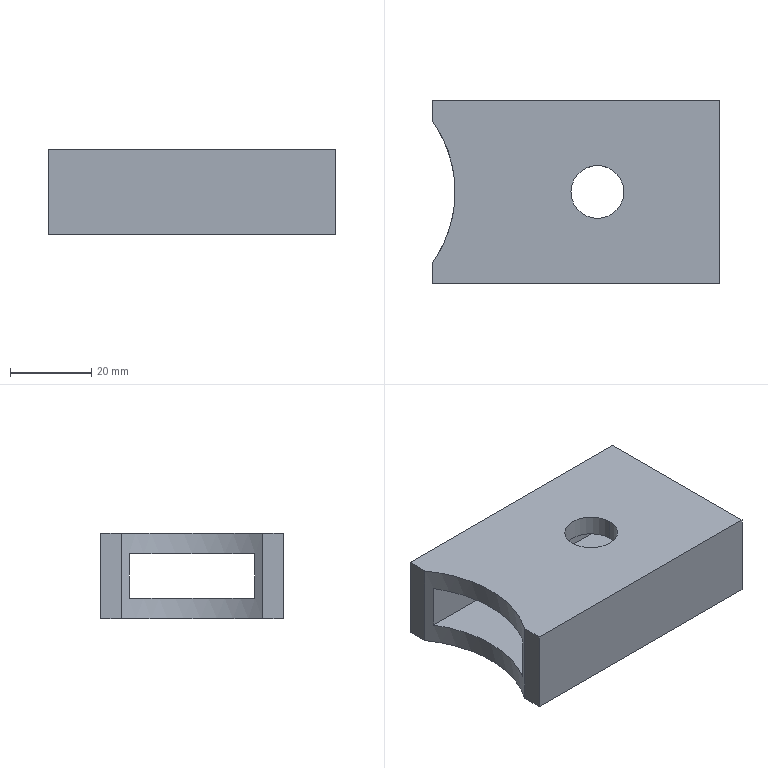Part | SolidWorks | features ICE 3, Extrusion 1 | 1 solid | 20 faces | box 70.526 x 45 x 21 mm | volume 38872 mm3 | plane 17 | cylinder 3 | commonest cylinder face diameters 13 x2 60 x1
STEP:
#1=CARTESIAN_POINT('',(71.5,0.,5.5));
#2=VERTEX_POINT('',#1);
#3=CARTESIAN_POINT('',(58.5,0.,5.5));
#4=VERTEX_POINT('',#3);
#5=CARTESIAN_POINT('',(65.,0.,5.5));
#6=DIRECTION('',(0.,0.,-1.));
#7=DIRECTION('',(0.,-1.,0.));
#8=AXIS2_PLACEMENT_3D('',#5,#6,#7);
#9=CIRCLE('',#8,6.5);
#10=EDGE_CURVE('',#2,#4,#9,.T.);
#11=ORIENTED_EDGE('',*,*,#10,.T.);
#12=CARTESIAN_POINT('',(58.5,0.,10.5));
#13=VERTEX_POINT('',#12);
#14=CARTESIAN_POINT('',(58.5,0.,-10.501));
#15=DIRECTION('',(0.,0.,1.));
#16=VECTOR('',#15,1000.);
#17=LINE('',#14,#16);
#18=EDGE_CURVE('',#4,#13,#17,.T.);
#19=ORIENTED_EDGE('',*,*,#18,.T.);
#20=CARTESIAN_POINT('',(71.5,0.,10.5));
#21=VERTEX_POINT('',#20);
#22=CARTESIAN_POINT('',(65.,0.,10.5));
#23=DIRECTION('',(0.,0.,1.));
#24=DIRECTION('',(1.,0.,0.));
#25=AXIS2_PLACEMENT_3D('',#22,#23,#24);
#26=CIRCLE('',#25,6.5);
#27=EDGE_CURVE('',#13,#21,#26,.T.);
#28=ORIENTED_EDGE('',*,*,#27,.T.);
#29=CARTESIAN_POINT('',(71.5,0.,-10.501));
#30=DIRECTION('',(0.,0.,1.));
#31=VECTOR('',#30,1000.);
#32=LINE('',#29,#31);
#33=EDGE_CURVE('',#2,#21,#32,.T.);
#34=ORIENTED_EDGE('',*,*,#33,.F.);
#35=EDGE_LOOP('',(#11,#19,#28,#34));
#36=FACE_OUTER_BOUND('',#35,.T.);
#37=CARTESIAN_POINT('',(65.,0.,-10.501));
#38=DIRECTION('',(0.,0.,1.));
#39=DIRECTION('',(1.,0.,0.));
#40=AXIS2_PLACEMENT_3D('',#37,#38,#39);
#41=CYLINDRICAL_SURFACE('',#40,6.5);
#42=ADVANCED_FACE('',(#36),#41,.F.);
#43=CARTESIAN_POINT('',(95.,22.5,-10.5));
#44=VERTEX_POINT('',#43);
#45=CARTESIAN_POINT('',(24.474,22.5,-10.5));
#46=VERTEX_POINT('',#45);
#47=CARTESIAN_POINT('',(24.474,22.5,-10.5));
#48=DIRECTION('',(-1.,0.,0.));
#49=VECTOR('',#48,1000.);
#50=LINE('',#47,#49);
#51=EDGE_CURVE('',#44,#46,#50,.T.);
#52=ORIENTED_EDGE('',*,*,#51,.T.);
#53=CARTESIAN_POINT('',(24.474,22.5,10.5));
#54=VERTEX_POINT('',#53);
#55=CARTESIAN_POINT('',(24.474,22.5,10.5));
#56=DIRECTION('',(0.,0.,-1.));
#57=VECTOR('',#56,1000.);
#58=LINE('',#55,#57);
#59=EDGE_CURVE('',#54,#46,#58,.T.);
#60=ORIENTED_EDGE('',*,*,#59,.F.);
#61=CARTESIAN_POINT('',(95.,22.5,10.5));
#62=VERTEX_POINT('',#61);
#63=CARTESIAN_POINT('',(24.474,22.5,10.5));
#64=DIRECTION('',(-1.,0.,0.));
#65=VECTOR('',#64,1000.);
#66=LINE('',#63,#65);
#67=EDGE_CURVE('',#62,#54,#66,.T.);
#68=ORIENTED_EDGE('',*,*,#67,.F.);
#69=CARTESIAN_POINT('',(95.,22.5,10.5));
#70=DIRECTION('',(0.,0.,-1.));
#71=VECTOR('',#70,1000.);
#72=LINE('',#69,#71);
#73=EDGE_CURVE('',#62,#44,#72,.T.);
#74=ORIENTED_EDGE('',*,*,#73,.T.);
#75=EDGE_LOOP('',(#52,#60,#68,#74));
#76=FACE_OUTER_BOUND('',#75,.T.);
#77=CARTESIAN_POINT('',(24.474,22.5,10.5));
#78=DIRECTION('',(0.,-1.,0.));
#79=DIRECTION('',(0.,0.,-1.));
#80=AXIS2_PLACEMENT_3D('',#77,#78,#79);
#81=PLANE('',#80);
#82=ADVANCED_FACE('',(#76),#81,.F.);
#83=CARTESIAN_POINT('',(24.474,17.35,-10.5));
#84=VERTEX_POINT('',#83);
#85=CARTESIAN_POINT('',(24.474,22.5,-10.5));
#86=DIRECTION('',(0.,-1.,0.));
#87=VECTOR('',#86,1000.);
#88=LINE('',#85,#87);
#89=EDGE_CURVE('',#46,#84,#88,.T.);
#90=ORIENTED_EDGE('',*,*,#89,.T.);
#91=CARTESIAN_POINT('',(24.474,17.35,10.5));
#92=VERTEX_POINT('',#91);
#93=CARTESIAN_POINT('',(24.474,17.35,10.5));
#94=DIRECTION('',(0.,0.,-1.));
#95=VECTOR('',#94,1000.);
#96=LINE('',#93,#95);
#97=EDGE_CURVE('',#92,#84,#96,.T.);
#98=ORIENTED_EDGE('',*,*,#97,.F.);
#99=CARTESIAN_POINT('',(24.474,22.5,10.5));
#100=DIRECTION('',(0.,-1.,0.));
#101=VECTOR('',#100,1000.);
#102=LINE('',#99,#101);
#103=EDGE_CURVE('',#54,#92,#102,.T.);
#104=ORIENTED_EDGE('',*,*,#103,.F.);
#105=ORIENTED_EDGE('',*,*,#59,.T.);
#106=EDGE_LOOP('',(#90,#98,#104,#105));
#107=FACE_OUTER_BOUND('',#106,.T.);
#108=CARTESIAN_POINT('',(24.474,22.5,10.5));
#109=DIRECTION('',(1.,0.,0.));
#110=DIRECTION('',(0.,1.,0.));
#111=AXIS2_PLACEMENT_3D('',#108,#109,#110);
#112=PLANE('',#111);
#113=ADVANCED_FACE('',(#107),#112,.F.);
#114=CARTESIAN_POINT('',(25.686,15.5,-5.5));
#115=VERTEX_POINT('',#114);
#116=CARTESIAN_POINT('',(25.686,15.5,5.5));
#117=VERTEX_POINT('',#116);
#118=CARTESIAN_POINT('',(25.686,15.5,10.5));
#119=DIRECTION('',(0.,0.,1.));
#120=VECTOR('',#119,1000.);
#121=LINE('',#118,#120);
#122=EDGE_CURVE('',#115,#117,#121,.T.);
#123=ORIENTED_EDGE('',*,*,#122,.T.);
#124=CARTESIAN_POINT('',(25.686,-15.5,5.5));
#125=VERTEX_POINT('',#124);
#126=CARTESIAN_POINT('',(0.,0.,5.5));
#127=DIRECTION('',(0.,0.,-1.));
#128=DIRECTION('',(0.,-1.,0.));
#129=AXIS2_PLACEMENT_3D('',#126,#127,#128);
#130=CIRCLE('',#129,30.);
#131=EDGE_CURVE('',#117,#125,#130,.T.);
#132=ORIENTED_EDGE('',*,*,#131,.T.);
#133=CARTESIAN_POINT('',(25.686,-15.5,-5.5));
#134=VERTEX_POINT('',#133);
#135=CARTESIAN_POINT('',(25.686,-15.5,10.5));
#136=DIRECTION('',(0.,0.,-1.));
#137=VECTOR('',#136,1000.);
#138=LINE('',#135,#137);
#139=EDGE_CURVE('',#125,#134,#138,.T.);
#140=ORIENTED_EDGE('',*,*,#139,.T.);
#141=CARTESIAN_POINT('',(0.,0.,-5.5));
#142=DIRECTION('',(0.,0.,1.));
#143=DIRECTION('',(0.,1.,0.));
#144=AXIS2_PLACEMENT_3D('',#141,#142,#143);
#145=CIRCLE('',#144,30.);
#146=EDGE_CURVE('',#134,#115,#145,.T.);
#147=ORIENTED_EDGE('',*,*,#146,.T.);
#148=EDGE_LOOP('',(#123,#132,#140,#147));
#149=FACE_BOUND('',#148,.T.);
#150=CARTESIAN_POINT('',(24.474,-17.35,-10.5));
#151=VERTEX_POINT('',#150);
#152=CARTESIAN_POINT('',(0.,0.,-10.5));
#153=DIRECTION('',(0.,0.,-1.));
#154=DIRECTION('',(-1.,0.,0.));
#155=AXIS2_PLACEMENT_3D('',#152,#153,#154);
#156=CIRCLE('',#155,30.);
#157=EDGE_CURVE('',#84,#151,#156,.T.);
#158=ORIENTED_EDGE('',*,*,#157,.T.);
#159=CARTESIAN_POINT('',(24.474,-17.35,10.5));
#160=VERTEX_POINT('',#159);
#161=CARTESIAN_POINT('',(24.474,-17.35,10.5));
#162=DIRECTION('',(0.,0.,-1.));
#163=VECTOR('',#162,1000.);
#164=LINE('',#161,#163);
#165=EDGE_CURVE('',#160,#151,#164,.T.);
#166=ORIENTED_EDGE('',*,*,#165,.F.);
#167=CARTESIAN_POINT('',(0.,0.,10.5));
#168=DIRECTION('',(0.,0.,-1.));
#169=DIRECTION('',(-1.,0.,0.));
#170=AXIS2_PLACEMENT_3D('',#167,#168,#169);
#171=CIRCLE('',#170,30.);
#172=EDGE_CURVE('',#92,#160,#171,.T.);
#173=ORIENTED_EDGE('',*,*,#172,.F.);
#174=ORIENTED_EDGE('',*,*,#97,.T.);
#175=EDGE_LOOP('',(#158,#166,#173,#174));
#176=FACE_OUTER_BOUND('',#175,.T.);
#177=CARTESIAN_POINT('',(0.,0.,10.5));
#178=DIRECTION('',(0.,0.,-1.));
#179=DIRECTION('',(-1.,0.,0.));
#180=AXIS2_PLACEMENT_3D('',#177,#178,#179);
#181=CYLINDRICAL_SURFACE('',#180,30.);
#182=ADVANCED_FACE('',(#149,#176),#181,.F.);
#183=CARTESIAN_POINT('',(24.474,-22.5,-10.5));
#184=VERTEX_POINT('',#183);
#185=CARTESIAN_POINT('',(24.474,-17.35,-10.5));
#186=DIRECTION('',(0.,-1.,0.));
#187=VECTOR('',#186,1000.);
#188=LINE('',#185,#187);
#189=EDGE_CURVE('',#151,#184,#188,.T.);
#190=ORIENTED_EDGE('',*,*,#189,.T.);
#191=CARTESIAN_POINT('',(24.474,-22.5,10.5));
#192=VERTEX_POINT('',#191);
#193=CARTESIAN_POINT('',(24.474,-22.5,10.5));
#194=DIRECTION('',(0.,0.,-1.));
#195=VECTOR('',#194,1000.);
#196=LINE('',#193,#195);
#197=EDGE_CURVE('',#192,#184,#196,.T.);
#198=ORIENTED_EDGE('',*,*,#197,.F.);
#199=CARTESIAN_POINT('',(24.474,-17.35,10.5));
#200=DIRECTION('',(0.,-1.,0.));
#201=VECTOR('',#200,1000.);
#202=LINE('',#199,#201);
#203=EDGE_CURVE('',#160,#192,#202,.T.);
#204=ORIENTED_EDGE('',*,*,#203,.F.);
#205=ORIENTED_EDGE('',*,*,#165,.T.);
#206=EDGE_LOOP('',(#190,#198,#204,#205));
#207=FACE_OUTER_BOUND('',#206,.T.);
#208=CARTESIAN_POINT('',(24.474,-17.35,10.5));
#209=DIRECTION('',(1.,0.,0.));
#210=DIRECTION('',(0.,1.,0.));
#211=AXIS2_PLACEMENT_3D('',#208,#209,#210);
#212=PLANE('',#211);
#213=ADVANCED_FACE('',(#207),#212,.F.);
#214=CARTESIAN_POINT('',(95.,-22.5,-10.5));
#215=VERTEX_POINT('',#214);
#216=CARTESIAN_POINT('',(24.474,-22.5,-10.5));
#217=DIRECTION('',(1.,0.,0.));
#218=VECTOR('',#217,1000.);
#219=LINE('',#216,#218);
#220=EDGE_CURVE('',#184,#215,#219,.T.);
#221=ORIENTED_EDGE('',*,*,#220,.T.);
#222=CARTESIAN_POINT('',(95.,-22.5,10.5));
#223=VERTEX_POINT('',#222);
#224=CARTESIAN_POINT('',(95.,-22.5,10.5));
#225=DIRECTION('',(0.,0.,-1.));
#226=VECTOR('',#225,1000.);
#227=LINE('',#224,#226);
#228=EDGE_CURVE('',#223,#215,#227,.T.);
#229=ORIENTED_EDGE('',*,*,#228,.F.);
#230=CARTESIAN_POINT('',(24.474,-22.5,10.5));
#231=DIRECTION('',(1.,0.,0.));
#232=VECTOR('',#231,1000.);
#233=LINE('',#230,#232);
#234=EDGE_CURVE('',#192,#223,#233,.T.);
#235=ORIENTED_EDGE('',*,*,#234,.F.);
#236=ORIENTED_EDGE('',*,*,#197,.T.);
#237=EDGE_LOOP('',(#221,#229,#235,#236));
#238=FACE_OUTER_BOUND('',#237,.T.);
#239=CARTESIAN_POINT('',(24.474,-22.5,10.5));
#240=DIRECTION('',(0.,1.,0.));
#241=DIRECTION('',(0.,0.,1.));
#242=AXIS2_PLACEMENT_3D('',#239,#240,#241);
#243=PLANE('',#242);
#244=ADVANCED_FACE('',(#238),#243,.F.);
#245=CARTESIAN_POINT('',(95.,-15.5,5.5));
#246=VERTEX_POINT('',#245);
#247=CARTESIAN_POINT('',(95.,-15.5,-5.5));
#248=VERTEX_POINT('',#247);
#249=CARTESIAN_POINT('',(95.,-15.5,5.5));
#250=DIRECTION('',(0.,0.,-1.));
#251=VECTOR('',#250,1000.);
#252=LINE('',#249,#251);
#253=EDGE_CURVE('',#246,#248,#252,.T.);
#254=ORIENTED_EDGE('',*,*,#253,.F.);
#255=CARTESIAN_POINT('',(95.,15.5,5.5));
#256=VERTEX_POINT('',#255);
#257=CARTESIAN_POINT('',(95.,15.5,5.5));
#258=DIRECTION('',(0.,-1.,0.));
#259=VECTOR('',#258,1000.);
#260=LINE('',#257,#259);
#261=EDGE_CURVE('',#256,#246,#260,.T.);
#262=ORIENTED_EDGE('',*,*,#261,.F.);
#263=CARTESIAN_POINT('',(95.,15.5,-5.5));
#264=VERTEX_POINT('',#263);
#265=CARTESIAN_POINT('',(95.,15.5,5.5));
#266=DIRECTION('',(0.,0.,1.));
#267=VECTOR('',#266,1000.);
#268=LINE('',#265,#267);
#269=EDGE_CURVE('',#264,#256,#268,.T.);
#270=ORIENTED_EDGE('',*,*,#269,.F.);
#271=CARTESIAN_POINT('',(95.,15.5,-5.5));
#272=DIRECTION('',(0.,1.,0.));
#273=VECTOR('',#272,1000.);
#274=LINE('',#271,#273);
#275=EDGE_CURVE('',#248,#264,#274,.T.);
#276=ORIENTED_EDGE('',*,*,#275,.F.);
#277=EDGE_LOOP('',(#254,#262,#270,#276));
#278=FACE_BOUND('',#277,.T.);
#279=CARTESIAN_POINT('',(95.,22.5,-10.5));
#280=DIRECTION('',(0.,1.,0.));
#281=VECTOR('',#280,1000.);
#282=LINE('',#279,#281);
#283=EDGE_CURVE('',#215,#44,#282,.T.);
#284=ORIENTED_EDGE('',*,*,#283,.T.);
#285=ORIENTED_EDGE('',*,*,#73,.F.);
#286=CARTESIAN_POINT('',(95.,22.5,10.5));
#287=DIRECTION('',(0.,1.,0.));
#288=VECTOR('',#287,1000.);
#289=LINE('',#286,#288);
#290=EDGE_CURVE('',#223,#62,#289,.T.);
#291=ORIENTED_EDGE('',*,*,#290,.F.);
#292=ORIENTED_EDGE('',*,*,#228,.T.);
#293=EDGE_LOOP('',(#284,#285,#291,#292));
#294=FACE_OUTER_BOUND('',#293,.T.);
#295=CARTESIAN_POINT('',(95.,22.5,10.5));
#296=DIRECTION('',(-1.,0.,0.));
#297=DIRECTION('',(0.,0.,1.));
#298=AXIS2_PLACEMENT_3D('',#295,#296,#297);
#299=PLANE('',#298);
#300=ADVANCED_FACE('',(#278,#294),#299,.F.);
#301=CARTESIAN_POINT('',(65.,0.,10.5));
#302=DIRECTION('',(0.,0.,1.));
#303=DIRECTION('',(1.,0.,0.));
#304=AXIS2_PLACEMENT_3D('',#301,#302,#303);
#305=CIRCLE('',#304,6.5);
#306=EDGE_CURVE('',#21,#13,#305,.T.);
#307=ORIENTED_EDGE('',*,*,#306,.F.);
#308=ORIENTED_EDGE('',*,*,#27,.F.);
#309=EDGE_LOOP('',(#307,#308));
#310=FACE_BOUND('',#309,.T.);
#311=ORIENTED_EDGE('',*,*,#67,.T.);
#312=ORIENTED_EDGE('',*,*,#103,.T.);
#313=ORIENTED_EDGE('',*,*,#172,.T.);
#314=ORIENTED_EDGE('',*,*,#203,.T.);
#315=ORIENTED_EDGE('',*,*,#234,.T.);
#316=ORIENTED_EDGE('',*,*,#290,.T.);
#317=EDGE_LOOP('',(#311,#312,#313,#314,#315,#316));
#318=FACE_OUTER_BOUND('',#317,.T.);
#319=CARTESIAN_POINT('',(0.,0.,10.5));
#320=DIRECTION('',(0.,0.,-1.));
#321=DIRECTION('',(-1.,0.,0.));
#322=AXIS2_PLACEMENT_3D('',#319,#320,#321);
#323=PLANE('',#322);
#324=ADVANCED_FACE('',(#310,#318),#323,.F.);
#325=CARTESIAN_POINT('',(70.779,-10.,-10.5));
#326=VERTEX_POINT('',#325);
#327=CARTESIAN_POINT('',(59.221,-10.,-10.5));
#328=VERTEX_POINT('',#327);
#329=CARTESIAN_POINT('',(0.,-10.,-10.5));
#330=DIRECTION('',(-1.,0.,0.));
#331=VECTOR('',#330,1000.);
#332=LINE('',#329,#331);
#333=EDGE_CURVE('',#326,#328,#332,.T.);
#334=ORIENTED_EDGE('',*,*,#333,.F.);
#335=CARTESIAN_POINT('',(76.55,0.,-10.5));
#336=VERTEX_POINT('',#335);
#337=CARTESIAN_POINT('',(57.427,-33.139,-10.5));
#338=DIRECTION('',(-0.4998,-0.8661,0.));
#339=VECTOR('',#338,1000.);
#340=LINE('',#337,#339);
#341=EDGE_CURVE('',#336,#326,#340,.T.);
#342=ORIENTED_EDGE('',*,*,#341,.F.);
#343=CARTESIAN_POINT('',(70.779,10.,-10.5));
#344=VERTEX_POINT('',#343);
#345=CARTESIAN_POINT('',(57.427,33.139,-10.5));
#346=DIRECTION('',(0.4998,-0.8661,0.));
#347=VECTOR('',#346,1000.);
#348=LINE('',#345,#347);
#349=EDGE_CURVE('',#344,#336,#348,.T.);
#350=ORIENTED_EDGE('',*,*,#349,.F.);
#351=CARTESIAN_POINT('',(59.221,10.,-10.5));
#352=VERTEX_POINT('',#351);
#353=CARTESIAN_POINT('',(0.,10.,-10.5));
#354=DIRECTION('',(-1.,0.,0.));
#355=VECTOR('',#354,1000.);
#356=LINE('',#353,#355);
#357=EDGE_CURVE('',#344,#352,#356,.T.);
#358=ORIENTED_EDGE('',*,*,#357,.T.);
#359=CARTESIAN_POINT('',(53.45,0.,-10.5));
#360=VERTEX_POINT('',#359);
#361=CARTESIAN_POINT('',(40.098,-23.139,-10.5));
#362=DIRECTION('',(-0.4998,-0.8661,0.));
#363=VECTOR('',#362,1000.);
#364=LINE('',#361,#363);
#365=EDGE_CURVE('',#352,#360,#364,.T.);
#366=ORIENTED_EDGE('',*,*,#365,.T.);
#367=CARTESIAN_POINT('',(40.098,23.139,-10.5));
#368=DIRECTION('',(0.4998,-0.8661,0.));
#369=VECTOR('',#368,1000.);
#370=LINE('',#367,#369);
#371=EDGE_CURVE('',#360,#328,#370,.T.);
#372=ORIENTED_EDGE('',*,*,#371,.T.);
#373=EDGE_LOOP('',(#334,#342,#350,#358,#366,#372));
#374=FACE_BOUND('',#373,.T.);
#375=ORIENTED_EDGE('',*,*,#51,.F.);
#376=ORIENTED_EDGE('',*,*,#283,.F.);
#377=ORIENTED_EDGE('',*,*,#220,.F.);
#378=ORIENTED_EDGE('',*,*,#189,.F.);
#379=ORIENTED_EDGE('',*,*,#157,.F.);
#380=ORIENTED_EDGE('',*,*,#89,.F.);
#381=EDGE_LOOP('',(#375,#376,#377,#378,#379,#380));
#382=FACE_OUTER_BOUND('',#381,.T.);
#383=CARTESIAN_POINT('',(0.,0.,-10.5));
#384=DIRECTION('',(0.,0.,-1.));
#385=DIRECTION('',(-1.,0.,0.));
#386=AXIS2_PLACEMENT_3D('',#383,#384,#385);
#387=PLANE('',#386);
#388=ADVANCED_FACE('',(#374,#382),#387,.T.);
#389=ORIENTED_EDGE('',*,*,#10,.F.);
#390=CARTESIAN_POINT('',(65.,0.,5.5));
#391=DIRECTION('',(0.,0.,-1.));
#392=DIRECTION('',(0.,-1.,0.));
#393=AXIS2_PLACEMENT_3D('',#390,#391,#392);
#394=CIRCLE('',#393,6.5);
#395=EDGE_CURVE('',#4,#2,#394,.T.);
#396=ORIENTED_EDGE('',*,*,#395,.F.);
#397=EDGE_LOOP('',(#389,#396));
#398=FACE_BOUND('',#397,.T.);
#399=CARTESIAN_POINT('',(24.474,15.5,5.5));
#400=DIRECTION('',(1.,0.,0.));
#401=VECTOR('',#400,1000.);
#402=LINE('',#399,#401);
#403=EDGE_CURVE('',#117,#256,#402,.T.);
#404=ORIENTED_EDGE('',*,*,#403,.T.);
#405=ORIENTED_EDGE('',*,*,#261,.T.);
#406=CARTESIAN_POINT('',(24.474,-15.5,5.5));
#407=DIRECTION('',(1.,0.,0.));
#408=VECTOR('',#407,1000.);
#409=LINE('',#406,#408);
#410=EDGE_CURVE('',#125,#246,#409,.T.);
#411=ORIENTED_EDGE('',*,*,#410,.F.);
#412=ORIENTED_EDGE('',*,*,#131,.F.);
#413=EDGE_LOOP('',(#404,#405,#411,#412));
#414=FACE_OUTER_BOUND('',#413,.T.);
#415=CARTESIAN_POINT('',(24.474,15.5,5.5));
#416=DIRECTION('',(0.,0.,1.));
#417=DIRECTION('',(0.,-1.,0.));
#418=AXIS2_PLACEMENT_3D('',#415,#416,#417);
#419=PLANE('',#418);
#420=ADVANCED_FACE('',(#398,#414),#419,.F.);
#421=CARTESIAN_POINT('',(24.474,15.5,-5.5));
#422=DIRECTION('',(1.,0.,0.));
#423=VECTOR('',#422,1000.);
#424=LINE('',#421,#423);
#425=EDGE_CURVE('',#115,#264,#424,.T.);
#426=ORIENTED_EDGE('',*,*,#425,.T.);
#427=ORIENTED_EDGE('',*,*,#269,.T.);
#428=ORIENTED_EDGE('',*,*,#403,.F.);
#429=ORIENTED_EDGE('',*,*,#122,.F.);
#430=EDGE_LOOP('',(#426,#427,#428,#429));
#431=FACE_OUTER_BOUND('',#430,.T.);
#432=CARTESIAN_POINT('',(24.474,15.5,5.5));
#433=DIRECTION('',(0.,1.,0.));
#434=DIRECTION('',(0.,0.,1.));
#435=AXIS2_PLACEMENT_3D('',#432,#433,#434);
#436=PLANE('',#435);
#437=ADVANCED_FACE('',(#431),#436,.F.);
#438=CARTESIAN_POINT('',(70.779,-10.,-5.5));
#439=VERTEX_POINT('',#438);
#440=CARTESIAN_POINT('',(76.55,0.,-5.5));
#441=VERTEX_POINT('',#440);
#442=CARTESIAN_POINT('',(57.427,-33.139,-5.5));
#443=DIRECTION('',(0.4998,0.8661,0.));
#444=VECTOR('',#443,1000.);
#445=LINE('',#442,#444);
#446=EDGE_CURVE('',#439,#441,#445,.T.);
#447=ORIENTED_EDGE('',*,*,#446,.F.);
#448=CARTESIAN_POINT('',(59.221,-10.,-5.5));
#449=VERTEX_POINT('',#448);
#450=CARTESIAN_POINT('',(0.,-10.,-5.5));
#451=DIRECTION('',(1.,0.,0.));
#452=VECTOR('',#451,1000.);
#453=LINE('',#450,#452);
#454=EDGE_CURVE('',#449,#439,#453,.T.);
#455=ORIENTED_EDGE('',*,*,#454,.F.);
#456=CARTESIAN_POINT('',(53.45,0.,-5.5));
#457=VERTEX_POINT('',#456);
#458=CARTESIAN_POINT('',(40.098,23.139,-5.5));
#459=DIRECTION('',(-0.4998,0.8661,0.));
#460=VECTOR('',#459,1000.);
#461=LINE('',#458,#460);
#462=EDGE_CURVE('',#449,#457,#461,.T.);
#463=ORIENTED_EDGE('',*,*,#462,.T.);
#464=CARTESIAN_POINT('',(59.221,10.,-5.5));
#465=VERTEX_POINT('',#464);
#466=CARTESIAN_POINT('',(40.098,-23.139,-5.5));
#467=DIRECTION('',(0.4998,0.8661,0.));
#468=VECTOR('',#467,1000.);
#469=LINE('',#466,#468);
#470=EDGE_CURVE('',#457,#465,#469,.T.);
#471=ORIENTED_EDGE('',*,*,#470,.T.);
#472=CARTESIAN_POINT('',(70.779,10.,-5.5));
#473=VERTEX_POINT('',#472);
#474=CARTESIAN_POINT('',(0.,10.,-5.5));
#475=DIRECTION('',(1.,0.,0.));
#476=VECTOR('',#475,1000.);
#477=LINE('',#474,#476);
#478=EDGE_CURVE('',#465,#473,#477,.T.);
#479=ORIENTED_EDGE('',*,*,#478,.T.);
#480=CARTESIAN_POINT('',(57.427,33.139,-5.5));
#481=DIRECTION('',(-0.4998,0.8661,0.));
#482=VECTOR('',#481,1000.);
#483=LINE('',#480,#482);
#484=EDGE_CURVE('',#441,#473,#483,.T.);
#485=ORIENTED_EDGE('',*,*,#484,.F.);
#486=EDGE_LOOP('',(#447,#455,#463,#471,#479,#485));
#487=FACE_BOUND('',#486,.T.);
#488=CARTESIAN_POINT('',(24.474,-15.5,-5.5));
#489=DIRECTION('',(1.,0.,0.));
#490=VECTOR('',#489,1000.);
#491=LINE('',#488,#490);
#492=EDGE_CURVE('',#134,#248,#491,.T.);
#493=ORIENTED_EDGE('',*,*,#492,.T.);
#494=ORIENTED_EDGE('',*,*,#275,.T.);
#495=ORIENTED_EDGE('',*,*,#425,.F.);
#496=ORIENTED_EDGE('',*,*,#146,.F.);
#497=EDGE_LOOP('',(#493,#494,#495,#496));
#498=FACE_OUTER_BOUND('',#497,.T.);
#499=CARTESIAN_POINT('',(24.474,15.5,-5.5));
#500=DIRECTION('',(0.,0.,-1.));
#501=DIRECTION('',(0.,1.,0.));
#502=AXIS2_PLACEMENT_3D('',#499,#500,#501);
#503=PLANE('',#502);
#504=ADVANCED_FACE('',(#487,#498),#503,.F.);
#505=ORIENTED_EDGE('',*,*,#410,.T.);
#506=ORIENTED_EDGE('',*,*,#253,.T.);
#507=ORIENTED_EDGE('',*,*,#492,.F.);
#508=ORIENTED_EDGE('',*,*,#139,.F.);
#509=EDGE_LOOP('',(#505,#506,#507,#508));
#510=FACE_OUTER_BOUND('',#509,.T.);
#511=CARTESIAN_POINT('',(24.474,-15.5,5.5));
#512=DIRECTION('',(0.,-1.,0.));
#513=DIRECTION('',(0.,0.,-1.));
#514=AXIS2_PLACEMENT_3D('',#511,#512,#513);
#515=PLANE('',#514);
#516=ADVANCED_FACE('',(#510),#515,.F.);
#517=ORIENTED_EDGE('',*,*,#18,.F.);
#518=ORIENTED_EDGE('',*,*,#395,.T.);
#519=ORIENTED_EDGE('',*,*,#33,.T.);
#520=ORIENTED_EDGE('',*,*,#306,.T.);
#521=EDGE_LOOP('',(#517,#518,#519,#520));
#522=FACE_OUTER_BOUND('',#521,.T.);
#523=CARTESIAN_POINT('',(65.,0.,-10.501));
#524=DIRECTION('',(0.,0.,1.));
#525=DIRECTION('',(1.,0.,0.));
#526=AXIS2_PLACEMENT_3D('',#523,#524,#525);
#527=CYLINDRICAL_SURFACE('',#526,6.5);
#528=ADVANCED_FACE('',(#522),#527,.F.);
#529=ORIENTED_EDGE('',*,*,#454,.T.);
#530=CARTESIAN_POINT('',(70.779,-10.,10.501));
#531=DIRECTION('',(0.,0.,-1.));
#532=VECTOR('',#531,1000.);
#533=LINE('',#530,#532);
#534=EDGE_CURVE('',#439,#326,#533,.T.);
#535=ORIENTED_EDGE('',*,*,#534,.T.);
#536=ORIENTED_EDGE('',*,*,#333,.T.);
#537=CARTESIAN_POINT('',(59.221,-10.,10.501));
#538=DIRECTION('',(0.,0.,-1.));
#539=VECTOR('',#538,1000.);
#540=LINE('',#537,#539);
#541=EDGE_CURVE('',#449,#328,#540,.T.);
#542=ORIENTED_EDGE('',*,*,#541,.F.);
#543=EDGE_LOOP('',(#529,#535,#536,#542));
#544=FACE_OUTER_BOUND('',#543,.T.);
#545=CARTESIAN_POINT('',(0.,-10.,10.501));
#546=DIRECTION('',(0.,-1.,0.));
#547=DIRECTION('',(0.,0.,-1.));
#548=AXIS2_PLACEMENT_3D('',#545,#546,#547);
#549=PLANE('',#548);
#550=ADVANCED_FACE('',(#544),#549,.F.);
#551=ORIENTED_EDGE('',*,*,#541,.T.);
#552=ORIENTED_EDGE('',*,*,#371,.F.);
#553=CARTESIAN_POINT('',(53.45,0.,10.501));
#554=DIRECTION('',(0.,0.,-1.));
#555=VECTOR('',#554,1000.);
#556=LINE('',#553,#555);
#557=EDGE_CURVE('',#457,#360,#556,.T.);
#558=ORIENTED_EDGE('',*,*,#557,.F.);
#559=ORIENTED_EDGE('',*,*,#462,.F.);
#560=EDGE_LOOP('',(#551,#552,#558,#559));
#561=FACE_OUTER_BOUND('',#560,.T.);
#562=CARTESIAN_POINT('',(40.098,23.139,10.501));
#563=DIRECTION('',(0.8661,0.4998,0.));
#564=DIRECTION('',(-0.4998,0.8661,0.));
#565=AXIS2_PLACEMENT_3D('',#562,#563,#564);
#566=PLANE('',#565);
#567=ADVANCED_FACE('',(#561),#566,.T.);
#568=ORIENTED_EDGE('',*,*,#557,.T.);
#569=ORIENTED_EDGE('',*,*,#365,.F.);
#570=CARTESIAN_POINT('',(59.221,10.,10.501));
#571=DIRECTION('',(0.,0.,-1.));
#572=VECTOR('',#571,1000.);
#573=LINE('',#570,#572);
#574=EDGE_CURVE('',#465,#352,#573,.T.);
#575=ORIENTED_EDGE('',*,*,#574,.F.);
#576=ORIENTED_EDGE('',*,*,#470,.F.);
#577=EDGE_LOOP('',(#568,#569,#575,#576));
#578=FACE_OUTER_BOUND('',#577,.T.);
#579=CARTESIAN_POINT('',(40.098,-23.139,10.501));
#580=DIRECTION('',(0.8661,-0.4998,0.));
#581=DIRECTION('',(0.4998,0.8661,0.));
#582=AXIS2_PLACEMENT_3D('',#579,#580,#581);
#583=PLANE('',#582);
#584=ADVANCED_FACE('',(#578),#583,.T.);
#585=ORIENTED_EDGE('',*,*,#574,.T.);
#586=ORIENTED_EDGE('',*,*,#357,.F.);
#587=CARTESIAN_POINT('',(70.779,10.,10.501));
#588=DIRECTION('',(0.,0.,-1.));
#589=VECTOR('',#588,1000.);
#590=LINE('',#587,#589);
#591=EDGE_CURVE('',#473,#344,#590,.T.);
#592=ORIENTED_EDGE('',*,*,#591,.F.);
#593=ORIENTED_EDGE('',*,*,#478,.F.);
#594=EDGE_LOOP('',(#585,#586,#592,#593));
#595=FACE_OUTER_BOUND('',#594,.T.);
#596=CARTESIAN_POINT('',(0.,10.,10.501));
#597=DIRECTION('',(0.,-1.,0.));
#598=DIRECTION('',(0.,0.,-1.));
#599=AXIS2_PLACEMENT_3D('',#596,#597,#598);
#600=PLANE('',#599);
#601=ADVANCED_FACE('',(#595),#600,.T.);
#602=ORIENTED_EDGE('',*,*,#484,.T.);
#603=ORIENTED_EDGE('',*,*,#591,.T.);
#604=ORIENTED_EDGE('',*,*,#349,.T.);
#605=CARTESIAN_POINT('',(76.55,0.,10.501));
#606=DIRECTION('',(0.,0.,-1.));
#607=VECTOR('',#606,1000.);
#608=LINE('',#605,#607);
#609=EDGE_CURVE('',#441,#336,#608,.T.);
#610=ORIENTED_EDGE('',*,*,#609,.F.);
#611=EDGE_LOOP('',(#602,#603,#604,#610));
#612=FACE_OUTER_BOUND('',#611,.T.);
#613=CARTESIAN_POINT('',(57.427,33.139,10.501));
#614=DIRECTION('',(0.8661,0.4998,0.));
#615=DIRECTION('',(-0.4998,0.8661,0.));
#616=AXIS2_PLACEMENT_3D('',#613,#614,#615);
#617=PLANE('',#616);
#618=ADVANCED_FACE('',(#612),#617,.F.);
#619=ORIENTED_EDGE('',*,*,#446,.T.);
#620=ORIENTED_EDGE('',*,*,#609,.T.);
#621=ORIENTED_EDGE('',*,*,#341,.T.);
#622=ORIENTED_EDGE('',*,*,#534,.F.);
#623=EDGE_LOOP('',(#619,#620,#621,#622));
#624=FACE_OUTER_BOUND('',#623,.T.);
#625=CARTESIAN_POINT('',(57.427,-33.139,10.501));
#626=DIRECTION('',(0.8661,-0.4998,0.));
#627=DIRECTION('',(0.4998,0.8661,0.));
#628=AXIS2_PLACEMENT_3D('',#625,#626,#627);
#629=PLANE('',#628);
#630=ADVANCED_FACE('',(#624),#629,.F.);
#631=CLOSED_SHELL('',(#42,#82,#113,#182,#213,#244,#300,#324,#388,#420,#437,#504,#516,#528,#550,#567,#584,#601,#618,#630));
#632=MANIFOLD_SOLID_BREP('',#631);
#633=CARTESIAN_POINT('',(0.,0.,0.));
#634=DIRECTION('',(0.,0.,1.));
#635=DIRECTION('',(1.,0.,0.));
#636=AXIS2_PLACEMENT_3D('',#633,#634,#635);
#637=(LENGTH_UNIT()NAMED_UNIT(*)SI_UNIT(.MILLI.,.METRE.));
#638=UNCERTAINTY_MEASURE_WITH_UNIT(LENGTH_MEASURE(0.00001),#637,'','');
#639=(NAMED_UNIT(*)PLANE_ANGLE_UNIT()SI_UNIT($,.RADIAN.));
#640=(NAMED_UNIT(*)SI_UNIT($,.STERADIAN.)SOLID_ANGLE_UNIT());
#641=(GEOMETRIC_REPRESENTATION_CONTEXT(3)GLOBAL_UNCERTAINTY_ASSIGNED_CONTEXT((#638))GLOBAL_UNIT_ASSIGNED_CONTEXT((#637,#639,#640))REPRESENTATION_CONTEXT('',''));
#642=ADVANCED_BREP_SHAPE_REPRESENTATION('',(#632,#636),#641);